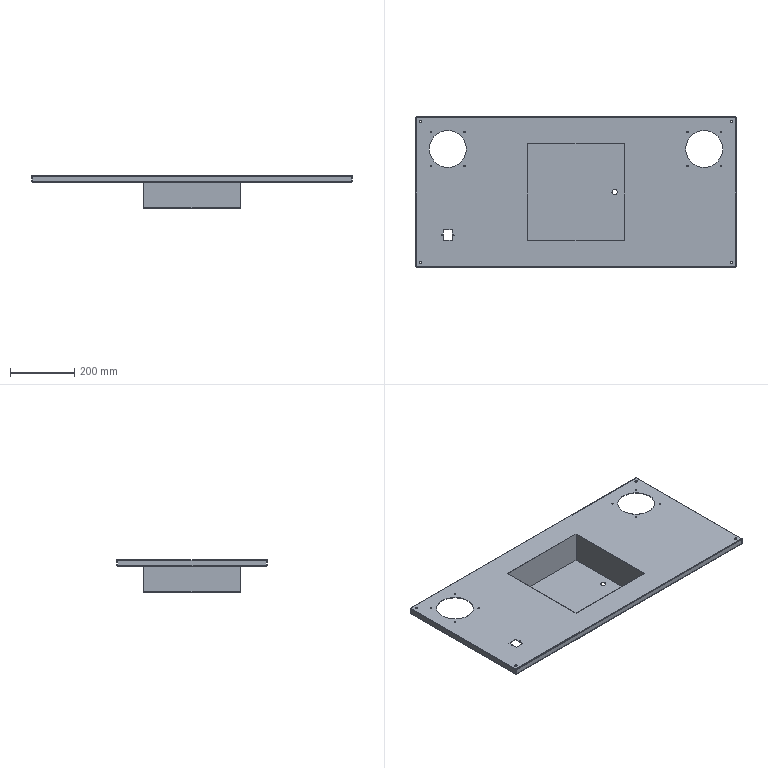Part | SolidWorks | features ICE 8, HoleWzd 3, EdgeFlange 2, FlatPattern 1, SMBaseFlange 1, SheetMetal 1 | 1 solid | 118 faces | box 998 x 468 x 101.5 mm | volume 960120 mm3 | plane 52 | cylinder 50 | spline 16 | commonest cylinder face diameters 5 x16 1.473 x8 4.473 x8 8 x8 2.5 x4 115 x4